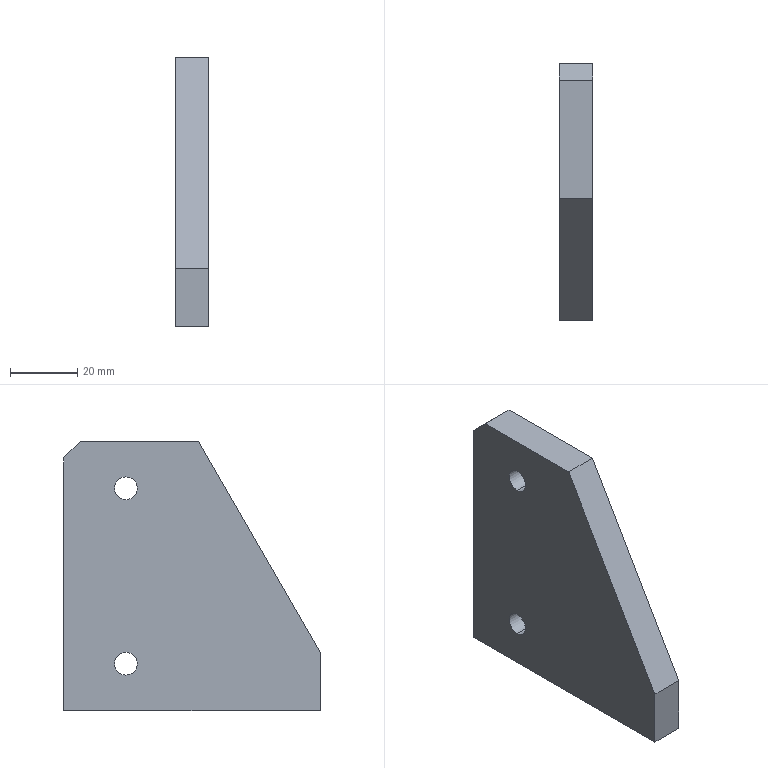Part | STEP file | X77-04207 | 1 solid | 12 faces | box 10 x 76.188 x 80 mm | volume 48758 mm3 | plane 8 | cylinder 4 | commonest cylinder face diameters 6.8 x4
STEP:
#1=CARTESIAN_POINT('',(-27.045,494.5,69.4));
#2=VERTEX_POINT('',#1);
#3=CARTESIAN_POINT('',(-27.045,494.5,62.6));
#4=VERTEX_POINT('',#3);
#5=CARTESIAN_POINT('',(-27.045,494.5,66.));
#6=DIRECTION('',(1.,0.,0.));
#7=DIRECTION('',(0.,0.,-1.));
#8=AXIS2_PLACEMENT_3D('',#5,#6,#7);
#9=CIRCLE('',#8,3.4);
#10=EDGE_CURVE('',#2,#4,#9,.T.);
#11=ORIENTED_EDGE('',*,*,#10,.F.);
#12=CARTESIAN_POINT('',(-17.045,494.5,69.4));
#13=VERTEX_POINT('',#12);
#14=CARTESIAN_POINT('',(-17.045,494.5,69.4));
#15=DIRECTION('',(1.,0.,0.));
#16=VECTOR('',#15,1000.);
#17=LINE('',#14,#16);
#18=EDGE_CURVE('',#2,#13,#17,.T.);
#19=ORIENTED_EDGE('',*,*,#18,.T.);
#20=CARTESIAN_POINT('',(-17.045,494.5,62.6));
#21=VERTEX_POINT('',#20);
#22=CARTESIAN_POINT('',(-17.045,494.5,66.));
#23=DIRECTION('',(1.,0.,0.));
#24=DIRECTION('',(0.,0.,-1.));
#25=AXIS2_PLACEMENT_3D('',#22,#23,#24);
#26=CIRCLE('',#25,3.4);
#27=EDGE_CURVE('',#13,#21,#26,.T.);
#28=ORIENTED_EDGE('',*,*,#27,.T.);
#29=CARTESIAN_POINT('',(-17.045,494.5,62.6));
#30=DIRECTION('',(1.,0.,0.));
#31=VECTOR('',#30,1000.);
#32=LINE('',#29,#31);
#33=EDGE_CURVE('',#4,#21,#32,.T.);
#34=ORIENTED_EDGE('',*,*,#33,.F.);
#35=EDGE_LOOP('',(#11,#19,#28,#34));
#36=FACE_OUTER_BOUND('',#35,.T.);
#37=CARTESIAN_POINT('',(-17.045,494.5,66.));
#38=DIRECTION('',(1.,0.,0.));
#39=DIRECTION('',(0.,0.,-1.));
#40=AXIS2_PLACEMENT_3D('',#37,#38,#39);
#41=CYLINDRICAL_SURFACE('',#40,3.4);
#42=ADVANCED_FACE('',(#36),#41,.F.);
#43=CARTESIAN_POINT('',(-27.045,494.5,17.4));
#44=VERTEX_POINT('',#43);
#45=CARTESIAN_POINT('',(-27.045,494.5,10.6));
#46=VERTEX_POINT('',#45);
#47=CARTESIAN_POINT('',(-27.045,494.5,14.));
#48=DIRECTION('',(1.,0.,0.));
#49=DIRECTION('',(0.,0.,-1.));
#50=AXIS2_PLACEMENT_3D('',#47,#48,#49);
#51=CIRCLE('',#50,3.4);
#52=EDGE_CURVE('',#44,#46,#51,.T.);
#53=ORIENTED_EDGE('',*,*,#52,.F.);
#54=CARTESIAN_POINT('',(-17.045,494.5,17.4));
#55=VERTEX_POINT('',#54);
#56=CARTESIAN_POINT('',(-17.045,494.5,17.4));
#57=DIRECTION('',(1.,0.,0.));
#58=VECTOR('',#57,1000.);
#59=LINE('',#56,#58);
#60=EDGE_CURVE('',#44,#55,#59,.T.);
#61=ORIENTED_EDGE('',*,*,#60,.T.);
#62=CARTESIAN_POINT('',(-17.045,494.5,10.6));
#63=VERTEX_POINT('',#62);
#64=CARTESIAN_POINT('',(-17.045,494.5,14.));
#65=DIRECTION('',(1.,0.,0.));
#66=DIRECTION('',(0.,0.,-1.));
#67=AXIS2_PLACEMENT_3D('',#64,#65,#66);
#68=CIRCLE('',#67,3.4);
#69=EDGE_CURVE('',#55,#63,#68,.T.);
#70=ORIENTED_EDGE('',*,*,#69,.T.);
#71=CARTESIAN_POINT('',(-17.045,494.5,10.6));
#72=DIRECTION('',(1.,0.,0.));
#73=VECTOR('',#72,1000.);
#74=LINE('',#71,#73);
#75=EDGE_CURVE('',#46,#63,#74,.T.);
#76=ORIENTED_EDGE('',*,*,#75,.F.);
#77=EDGE_LOOP('',(#53,#61,#70,#76));
#78=FACE_OUTER_BOUND('',#77,.T.);
#79=CARTESIAN_POINT('',(-17.045,494.5,14.));
#80=DIRECTION('',(1.,0.,0.));
#81=DIRECTION('',(0.,0.,-1.));
#82=AXIS2_PLACEMENT_3D('',#79,#80,#81);
#83=CYLINDRICAL_SURFACE('',#82,3.4);
#84=ADVANCED_FACE('',(#78),#83,.F.);
#85=CARTESIAN_POINT('',(-17.045,494.5,66.));
#86=DIRECTION('',(1.,0.,0.));
#87=DIRECTION('',(0.,0.,-1.));
#88=AXIS2_PLACEMENT_3D('',#85,#86,#87);
#89=CIRCLE('',#88,3.4);
#90=EDGE_CURVE('',#21,#13,#89,.T.);
#91=ORIENTED_EDGE('',*,*,#90,.F.);
#92=ORIENTED_EDGE('',*,*,#27,.F.);
#93=EDGE_LOOP('',(#91,#92));
#94=FACE_BOUND('',#93,.T.);
#95=CARTESIAN_POINT('',(-17.045,494.5,14.));
#96=DIRECTION('',(1.,0.,0.));
#97=DIRECTION('',(0.,0.,-1.));
#98=AXIS2_PLACEMENT_3D('',#95,#96,#97);
#99=CIRCLE('',#98,3.4);
#100=EDGE_CURVE('',#63,#55,#99,.T.);
#101=ORIENTED_EDGE('',*,*,#100,.F.);
#102=ORIENTED_EDGE('',*,*,#69,.F.);
#103=EDGE_LOOP('',(#101,#102));
#104=FACE_BOUND('',#103,.T.);
#105=CARTESIAN_POINT('',(-17.045,513.,75.));
#106=VERTEX_POINT('',#105);
#107=CARTESIAN_POINT('',(-17.045,513.,0.));
#108=VERTEX_POINT('',#107);
#109=CARTESIAN_POINT('',(-17.045,513.,80.));
#110=DIRECTION('',(0.,0.,-1.));
#111=VECTOR('',#110,1000.);
#112=LINE('',#109,#111);
#113=EDGE_CURVE('',#106,#108,#112,.T.);
#114=ORIENTED_EDGE('',*,*,#113,.F.);
#115=CARTESIAN_POINT('',(-17.045,508.,80.));
#116=VERTEX_POINT('',#115);
#117=CARTESIAN_POINT('',(-17.045,508.,80.));
#118=DIRECTION('',(0.,-0.7071,0.7071));
#119=VECTOR('',#118,1000.);
#120=LINE('',#117,#119);
#121=EDGE_CURVE('',#106,#116,#120,.T.);
#122=ORIENTED_EDGE('',*,*,#121,.T.);
#123=CARTESIAN_POINT('',(-17.045,473.,80.));
#124=VERTEX_POINT('',#123);
#125=CARTESIAN_POINT('',(-17.045,513.,80.));
#126=DIRECTION('',(0.,1.,0.));
#127=VECTOR('',#126,1000.);
#128=LINE('',#125,#127);
#129=EDGE_CURVE('',#124,#116,#128,.T.);
#130=ORIENTED_EDGE('',*,*,#129,.F.);
#131=CARTESIAN_POINT('',(-17.045,436.812,17.321));
#132=VERTEX_POINT('',#131);
#133=CARTESIAN_POINT('',(-17.045,473.,80.));
#134=DIRECTION('',(0.,-0.5,-0.866));
#135=VECTOR('',#134,1000.);
#136=LINE('',#133,#135);
#137=EDGE_CURVE('',#124,#132,#136,.T.);
#138=ORIENTED_EDGE('',*,*,#137,.T.);
#139=CARTESIAN_POINT('',(-17.045,436.812,0.));
#140=VERTEX_POINT('',#139);
#141=CARTESIAN_POINT('',(-17.045,436.812,0.));
#142=DIRECTION('',(0.,0.,-1.));
#143=VECTOR('',#142,1000.);
#144=LINE('',#141,#143);
#145=EDGE_CURVE('',#132,#140,#144,.T.);
#146=ORIENTED_EDGE('',*,*,#145,.T.);
#147=CARTESIAN_POINT('',(-17.045,513.,0.));
#148=DIRECTION('',(0.,1.,0.));
#149=VECTOR('',#148,1000.);
#150=LINE('',#147,#149);
#151=EDGE_CURVE('',#140,#108,#150,.T.);
#152=ORIENTED_EDGE('',*,*,#151,.T.);
#153=EDGE_LOOP('',(#114,#122,#130,#138,#146,#152));
#154=FACE_OUTER_BOUND('',#153,.T.);
#155=CARTESIAN_POINT('',(-17.045,513.,80.));
#156=DIRECTION('',(-1.,0.,0.));
#157=DIRECTION('',(0.,-1.,0.));
#158=AXIS2_PLACEMENT_3D('',#155,#156,#157);
#159=PLANE('',#158);
#160=ADVANCED_FACE('',(#94,#104,#154),#159,.F.);
#161=CARTESIAN_POINT('',(-27.045,513.,75.));
#162=VERTEX_POINT('',#161);
#163=CARTESIAN_POINT('',(-27.045,513.,0.));
#164=VERTEX_POINT('',#163);
#165=CARTESIAN_POINT('',(-27.045,513.,80.));
#166=DIRECTION('',(0.,0.,-1.));
#167=VECTOR('',#166,1000.);
#168=LINE('',#165,#167);
#169=EDGE_CURVE('',#162,#164,#168,.T.);
#170=ORIENTED_EDGE('',*,*,#169,.F.);
#171=CARTESIAN_POINT('',(-17.045,513.,75.));
#172=DIRECTION('',(1.,0.,0.));
#173=VECTOR('',#172,1000.);
#174=LINE('',#171,#173);
#175=EDGE_CURVE('',#162,#106,#174,.T.);
#176=ORIENTED_EDGE('',*,*,#175,.T.);
#177=ORIENTED_EDGE('',*,*,#113,.T.);
#178=CARTESIAN_POINT('',(-17.045,513.,0.));
#179=DIRECTION('',(-1.,0.,0.));
#180=VECTOR('',#179,1000.);
#181=LINE('',#178,#180);
#182=EDGE_CURVE('',#108,#164,#181,.T.);
#183=ORIENTED_EDGE('',*,*,#182,.T.);
#184=EDGE_LOOP('',(#170,#176,#177,#183));
#185=FACE_OUTER_BOUND('',#184,.T.);
#186=CARTESIAN_POINT('',(-17.045,513.,80.));
#187=DIRECTION('',(0.,-1.,0.));
#188=DIRECTION('',(0.,0.,-1.));
#189=AXIS2_PLACEMENT_3D('',#186,#187,#188);
#190=PLANE('',#189);
#191=ADVANCED_FACE('',(#185),#190,.F.);
#192=CARTESIAN_POINT('',(-27.045,494.5,66.));
#193=DIRECTION('',(1.,0.,0.));
#194=DIRECTION('',(0.,0.,-1.));
#195=AXIS2_PLACEMENT_3D('',#192,#193,#194);
#196=CIRCLE('',#195,3.4);
#197=EDGE_CURVE('',#4,#2,#196,.T.);
#198=ORIENTED_EDGE('',*,*,#197,.T.);
#199=ORIENTED_EDGE('',*,*,#10,.T.);
#200=EDGE_LOOP('',(#198,#199));
#201=FACE_BOUND('',#200,.T.);
#202=CARTESIAN_POINT('',(-27.045,494.5,14.));
#203=DIRECTION('',(1.,0.,0.));
#204=DIRECTION('',(0.,0.,-1.));
#205=AXIS2_PLACEMENT_3D('',#202,#203,#204);
#206=CIRCLE('',#205,3.4);
#207=EDGE_CURVE('',#46,#44,#206,.T.);
#208=ORIENTED_EDGE('',*,*,#207,.T.);
#209=ORIENTED_EDGE('',*,*,#52,.T.);
#210=EDGE_LOOP('',(#208,#209));
#211=FACE_BOUND('',#210,.T.);
#212=CARTESIAN_POINT('',(-27.045,508.,80.));
#213=VERTEX_POINT('',#212);
#214=CARTESIAN_POINT('',(-27.045,473.,80.));
#215=VERTEX_POINT('',#214);
#216=CARTESIAN_POINT('',(-27.045,513.,80.));
#217=DIRECTION('',(0.,-1.,0.));
#218=VECTOR('',#217,1000.);
#219=LINE('',#216,#218);
#220=EDGE_CURVE('',#213,#215,#219,.T.);
#221=ORIENTED_EDGE('',*,*,#220,.F.);
#222=CARTESIAN_POINT('',(-27.045,508.,80.));
#223=DIRECTION('',(0.,0.7071,-0.7071));
#224=VECTOR('',#223,1000.);
#225=LINE('',#222,#224);
#226=EDGE_CURVE('',#213,#162,#225,.T.);
#227=ORIENTED_EDGE('',*,*,#226,.T.);
#228=ORIENTED_EDGE('',*,*,#169,.T.);
#229=CARTESIAN_POINT('',(-27.045,436.812,0.));
#230=VERTEX_POINT('',#229);
#231=CARTESIAN_POINT('',(-27.045,513.,0.));
#232=DIRECTION('',(0.,-1.,0.));
#233=VECTOR('',#232,1000.);
#234=LINE('',#231,#233);
#235=EDGE_CURVE('',#164,#230,#234,.T.);
#236=ORIENTED_EDGE('',*,*,#235,.T.);
#237=CARTESIAN_POINT('',(-27.045,436.812,17.321));
#238=VERTEX_POINT('',#237);
#239=CARTESIAN_POINT('',(-27.045,436.812,0.));
#240=DIRECTION('',(0.,0.,1.));
#241=VECTOR('',#240,1000.);
#242=LINE('',#239,#241);
#243=EDGE_CURVE('',#230,#238,#242,.T.);
#244=ORIENTED_EDGE('',*,*,#243,.T.);
#245=CARTESIAN_POINT('',(-27.045,473.,80.));
#246=DIRECTION('',(0.,0.5,0.866));
#247=VECTOR('',#246,1000.);
#248=LINE('',#245,#247);
#249=EDGE_CURVE('',#238,#215,#248,.T.);
#250=ORIENTED_EDGE('',*,*,#249,.T.);
#251=EDGE_LOOP('',(#221,#227,#228,#236,#244,#250));
#252=FACE_OUTER_BOUND('',#251,.T.);
#253=CARTESIAN_POINT('',(-27.045,513.,80.));
#254=DIRECTION('',(1.,0.,0.));
#255=DIRECTION('',(0.,0.,-1.));
#256=AXIS2_PLACEMENT_3D('',#253,#254,#255);
#257=PLANE('',#256);
#258=ADVANCED_FACE('',(#201,#211,#252),#257,.F.);
#259=ORIENTED_EDGE('',*,*,#129,.T.);
#260=CARTESIAN_POINT('',(-17.045,508.,80.));
#261=DIRECTION('',(-1.,0.,0.));
#262=VECTOR('',#261,1000.);
#263=LINE('',#260,#262);
#264=EDGE_CURVE('',#116,#213,#263,.T.);
#265=ORIENTED_EDGE('',*,*,#264,.T.);
#266=ORIENTED_EDGE('',*,*,#220,.T.);
#267=CARTESIAN_POINT('',(-17.045,473.,80.));
#268=DIRECTION('',(1.,0.,0.));
#269=VECTOR('',#268,1000.);
#270=LINE('',#267,#269);
#271=EDGE_CURVE('',#215,#124,#270,.T.);
#272=ORIENTED_EDGE('',*,*,#271,.T.);
#273=EDGE_LOOP('',(#259,#265,#266,#272));
#274=FACE_OUTER_BOUND('',#273,.T.);
#275=CARTESIAN_POINT('',(-17.045,473.,80.));
#276=DIRECTION('',(0.,0.,-1.));
#277=DIRECTION('',(-1.,0.,0.));
#278=AXIS2_PLACEMENT_3D('',#275,#276,#277);
#279=PLANE('',#278);
#280=ADVANCED_FACE('',(#274),#279,.F.);
#281=ORIENTED_EDGE('',*,*,#151,.F.);
#282=CARTESIAN_POINT('',(-114.849,436.812,0.));
#283=DIRECTION('',(1.,0.,0.));
#284=VECTOR('',#283,1000.);
#285=LINE('',#282,#284);
#286=EDGE_CURVE('',#230,#140,#285,.T.);
#287=ORIENTED_EDGE('',*,*,#286,.F.);
#288=ORIENTED_EDGE('',*,*,#235,.F.);
#289=ORIENTED_EDGE('',*,*,#182,.F.);
#290=EDGE_LOOP('',(#281,#287,#288,#289));
#291=FACE_OUTER_BOUND('',#290,.T.);
#292=CARTESIAN_POINT('',(-17.045,473.,0.));
#293=DIRECTION('',(0.,0.,-1.));
#294=DIRECTION('',(-1.,0.,0.));
#295=AXIS2_PLACEMENT_3D('',#292,#293,#294);
#296=PLANE('',#295);
#297=ADVANCED_FACE('',(#291),#296,.T.);
#298=ORIENTED_EDGE('',*,*,#243,.F.);
#299=ORIENTED_EDGE('',*,*,#286,.T.);
#300=ORIENTED_EDGE('',*,*,#145,.F.);
#301=CARTESIAN_POINT('',(-114.849,436.812,17.321));
#302=DIRECTION('',(1.,0.,0.));
#303=VECTOR('',#302,1000.);
#304=LINE('',#301,#303);
#305=EDGE_CURVE('',#238,#132,#304,.T.);
#306=ORIENTED_EDGE('',*,*,#305,.F.);
#307=EDGE_LOOP('',(#298,#299,#300,#306));
#308=FACE_OUTER_BOUND('',#307,.T.);
#309=CARTESIAN_POINT('',(-114.849,436.812,0.));
#310=DIRECTION('',(0.,-1.,0.));
#311=DIRECTION('',(1.,0.,0.));
#312=AXIS2_PLACEMENT_3D('',#309,#310,#311);
#313=PLANE('',#312);
#314=ADVANCED_FACE('',(#308),#313,.T.);
#315=ORIENTED_EDGE('',*,*,#249,.F.);
#316=ORIENTED_EDGE('',*,*,#305,.T.);
#317=ORIENTED_EDGE('',*,*,#137,.F.);
#318=ORIENTED_EDGE('',*,*,#271,.F.);
#319=EDGE_LOOP('',(#315,#316,#317,#318));
#320=FACE_OUTER_BOUND('',#319,.T.);
#321=CARTESIAN_POINT('',(-114.849,473.,80.));
#322=DIRECTION('',(0.,-0.866,0.5));
#323=DIRECTION('',(0.,-0.5,-0.866));
#324=AXIS2_PLACEMENT_3D('',#321,#322,#323);
#325=PLANE('',#324);
#326=ADVANCED_FACE('',(#320),#325,.T.);
#327=ORIENTED_EDGE('',*,*,#60,.F.);
#328=ORIENTED_EDGE('',*,*,#207,.F.);
#329=ORIENTED_EDGE('',*,*,#75,.T.);
#330=ORIENTED_EDGE('',*,*,#100,.T.);
#331=EDGE_LOOP('',(#327,#328,#329,#330));
#332=FACE_OUTER_BOUND('',#331,.T.);
#333=CARTESIAN_POINT('',(-17.045,494.5,14.));
#334=DIRECTION('',(1.,0.,0.));
#335=DIRECTION('',(0.,0.,-1.));
#336=AXIS2_PLACEMENT_3D('',#333,#334,#335);
#337=CYLINDRICAL_SURFACE('',#336,3.4);
#338=ADVANCED_FACE('',(#332),#337,.F.);
#339=ORIENTED_EDGE('',*,*,#18,.F.);
#340=ORIENTED_EDGE('',*,*,#197,.F.);
#341=ORIENTED_EDGE('',*,*,#33,.T.);
#342=ORIENTED_EDGE('',*,*,#90,.T.);
#343=EDGE_LOOP('',(#339,#340,#341,#342));
#344=FACE_OUTER_BOUND('',#343,.T.);
#345=CARTESIAN_POINT('',(-17.045,494.5,66.));
#346=DIRECTION('',(1.,0.,0.));
#347=DIRECTION('',(0.,0.,-1.));
#348=AXIS2_PLACEMENT_3D('',#345,#346,#347);
#349=CYLINDRICAL_SURFACE('',#348,3.4);
#350=ADVANCED_FACE('',(#344),#349,.F.);
#351=ORIENTED_EDGE('',*,*,#121,.F.);
#352=ORIENTED_EDGE('',*,*,#175,.F.);
#353=ORIENTED_EDGE('',*,*,#226,.F.);
#354=ORIENTED_EDGE('',*,*,#264,.F.);
#355=EDGE_LOOP('',(#351,#352,#353,#354));
#356=FACE_OUTER_BOUND('',#355,.T.);
#357=CARTESIAN_POINT('',(-17.045,508.,80.));
#358=DIRECTION('',(0.,-0.7071,-0.7071));
#359=DIRECTION('',(0.,0.7071,-0.7071));
#360=AXIS2_PLACEMENT_3D('',#357,#358,#359);
#361=PLANE('',#360);
#362=ADVANCED_FACE('',(#356),#361,.F.);
#363=CLOSED_SHELL('',(#42,#84,#160,#191,#258,#280,#297,#314,#326,#338,#350,#362));
#364=MANIFOLD_SOLID_BREP('',#363);
#365=CARTESIAN_POINT('',(0.,0.,0.));
#366=DIRECTION('',(0.,0.,1.));
#367=DIRECTION('',(1.,0.,0.));
#368=AXIS2_PLACEMENT_3D('',#365,#366,#367);
#369=(LENGTH_UNIT()NAMED_UNIT(*)SI_UNIT(.MILLI.,.METRE.));
#370=UNCERTAINTY_MEASURE_WITH_UNIT(LENGTH_MEASURE(0.00001),#369,'','');
#371=(NAMED_UNIT(*)PLANE_ANGLE_UNIT()SI_UNIT($,.RADIAN.));
#372=(NAMED_UNIT(*)SI_UNIT($,.STERADIAN.)SOLID_ANGLE_UNIT());
#373=(GEOMETRIC_REPRESENTATION_CONTEXT(3)GLOBAL_UNCERTAINTY_ASSIGNED_CONTEXT((#370))GLOBAL_UNIT_ASSIGNED_CONTEXT((#369,#371,#372))REPRESENTATION_CONTEXT('',''));
#374=ADVANCED_BREP_SHAPE_REPRESENTATION('',(#364,#368),#373);